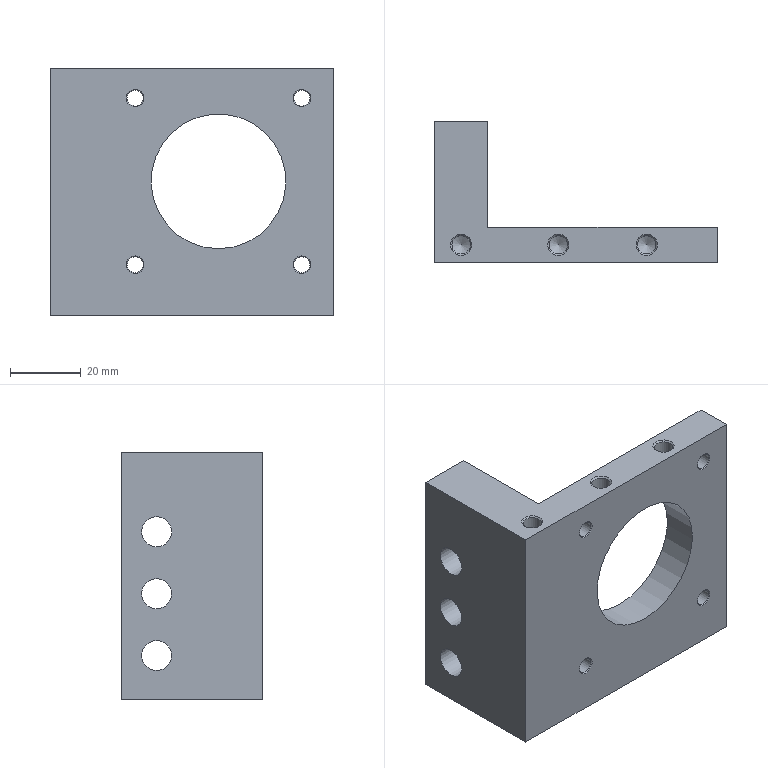Part | NX | features SIMPLE HOLE 8, SYMBOLIC_THREAD 7, DATUM_CSYS 6, SKETCH 5, HOLE PACKAGE 4, CBORE_HOLE 3, EXTRUDE 3 | 1 solid | 39 faces | box 80 x 40 x 70 mm | volume 69498 mm3 | cylinder 14 | cone 14 | plane 11 | commonest cylinder face diameters 4.5 x4 5.2 x3 8.5 x3 14 x3 38.1 x1
STEP:
#1=CARTESIAN_POINT('',(80.,10.,0.));
#2=VERTEX_POINT('',#1);
#3=CARTESIAN_POINT('',(15.,10.,0.));
#4=VERTEX_POINT('',#3);
#5=CARTESIAN_POINT('',(80.,10.,0.));
#6=DIRECTION('',(-1.,0.,0.));
#7=VECTOR('',#6,1000.);
#8=LINE('',#5,#7);
#9=EDGE_CURVE('',#2,#4,#8,.T.);
#10=ORIENTED_EDGE('',*,*,#9,.F.);
#11=CARTESIAN_POINT('',(80.,0.,0.));
#12=VERTEX_POINT('',#11);
#13=CARTESIAN_POINT('',(80.,0.,0.));
#14=DIRECTION('',(0.,-1.,0.));
#15=VECTOR('',#14,1000.);
#16=LINE('',#13,#15);
#17=EDGE_CURVE('',#12,#2,#16,.F.);
#18=ORIENTED_EDGE('',*,*,#17,.F.);
#19=CARTESIAN_POINT('',(0.,0.,0.));
#20=VERTEX_POINT('',#19);
#21=CARTESIAN_POINT('',(0.,0.,0.));
#22=DIRECTION('',(1.,0.,0.));
#23=VECTOR('',#22,1000.);
#24=LINE('',#21,#23);
#25=EDGE_CURVE('',#20,#12,#24,.T.);
#26=ORIENTED_EDGE('',*,*,#25,.F.);
#27=CARTESIAN_POINT('',(0.,40.,0.));
#28=VERTEX_POINT('',#27);
#29=CARTESIAN_POINT('',(0.,40.,0.));
#30=DIRECTION('',(0.,-1.,0.));
#31=VECTOR('',#30,1000.);
#32=LINE('',#29,#31);
#33=EDGE_CURVE('',#28,#20,#32,.T.);
#34=ORIENTED_EDGE('',*,*,#33,.F.);
#35=CARTESIAN_POINT('',(15.,40.,0.));
#36=VERTEX_POINT('',#35);
#37=CARTESIAN_POINT('',(0.,40.,0.));
#38=DIRECTION('',(-1.,0.,0.));
#39=VECTOR('',#38,1000.);
#40=LINE('',#37,#39);
#41=EDGE_CURVE('',#28,#36,#40,.F.);
#42=ORIENTED_EDGE('',*,*,#41,.T.);
#43=CARTESIAN_POINT('',(15.,40.,0.));
#44=DIRECTION('',(0.,-1.,0.));
#45=VECTOR('',#44,1000.);
#46=LINE('',#43,#45);
#47=EDGE_CURVE('',#36,#4,#46,.T.);
#48=ORIENTED_EDGE('',*,*,#47,.T.);
#49=EDGE_LOOP('',(#10,#18,#26,#34,#42,#48));
#50=FACE_BOUND('',#49,.T.);
#51=CARTESIAN_POINT('',(0.,0.,0.));
#52=DIRECTION('',(0.,0.,-1.));
#53=DIRECTION('',(1.,0.,0.));
#54=AXIS2_PLACEMENT_3D('',#51,#52,#53);
#55=PLANE('',#54);
#56=ADVANCED_FACE('',(#50),#55,.T.);
#57=CARTESIAN_POINT('',(80.,10.,70.));
#58=VERTEX_POINT('',#57);
#59=CARTESIAN_POINT('',(80.,10.,60.));
#60=DIRECTION('',(0.,0.,-1.));
#61=VECTOR('',#60,1000.);
#62=LINE('',#59,#61);
#63=EDGE_CURVE('',#58,#2,#62,.T.);
#64=ORIENTED_EDGE('',*,*,#63,.F.);
#65=CARTESIAN_POINT('',(80.,0.,70.));
#66=VERTEX_POINT('',#65);
#67=CARTESIAN_POINT('',(80.,0.,70.));
#68=DIRECTION('',(0.,1.,0.));
#69=VECTOR('',#68,1000.);
#70=LINE('',#67,#69);
#71=EDGE_CURVE('',#66,#58,#70,.T.);
#72=ORIENTED_EDGE('',*,*,#71,.F.);
#73=CARTESIAN_POINT('',(80.,0.,0.));
#74=DIRECTION('',(0.,0.,1.));
#75=VECTOR('',#74,1000.);
#76=LINE('',#73,#75);
#77=EDGE_CURVE('',#12,#66,#76,.T.);
#78=ORIENTED_EDGE('',*,*,#77,.F.);
#79=ORIENTED_EDGE('',*,*,#17,.T.);
#80=EDGE_LOOP('',(#64,#72,#78,#79));
#81=FACE_BOUND('',#80,.T.);
#82=CARTESIAN_POINT('',(80.,0.,0.));
#83=DIRECTION('',(1.,0.,0.));
#84=DIRECTION('',(0.,0.,1.));
#85=AXIS2_PLACEMENT_3D('',#82,#83,#84);
#86=PLANE('',#85);
#87=ADVANCED_FACE('',(#81),#86,.T.);
#88=CARTESIAN_POINT('',(47.5,0.,18.95));
#89=VERTEX_POINT('',#88);
#90=CARTESIAN_POINT('',(47.5,0.,38.));
#91=DIRECTION('',(0.,-1.,0.));
#92=DIRECTION('',(0.,0.,-1.));
#93=AXIS2_PLACEMENT_3D('',#90,#91,#92);
#94=CIRCLE('',#93,19.05);
#95=EDGE_CURVE('',#89,#89,#94,.T.);
#96=ORIENTED_EDGE('',*,*,#95,.T.);
#97=EDGE_LOOP('',(#96));
#98=FACE_BOUND('',#97,.T.);
#99=CARTESIAN_POINT('',(47.5,10.,18.95));
#100=VERTEX_POINT('',#99);
#101=CARTESIAN_POINT('',(47.5,10.,38.));
#102=DIRECTION('',(0.,-1.,0.));
#103=DIRECTION('',(0.,0.,-1.));
#104=AXIS2_PLACEMENT_3D('',#101,#102,#103);
#105=CIRCLE('',#104,19.05);
#106=EDGE_CURVE('',#100,#100,#105,.T.);
#107=ORIENTED_EDGE('',*,*,#106,.F.);
#108=EDGE_LOOP('',(#107));
#109=FACE_BOUND('',#108,.T.);
#110=CARTESIAN_POINT('',(47.5,15.,38.));
#111=DIRECTION('',(0.,-1.,0.));
#112=DIRECTION('',(0.,0.,-1.));
#113=AXIS2_PLACEMENT_3D('',#110,#111,#112);
#114=CYLINDRICAL_SURFACE('',#113,19.05);
#115=ADVANCED_FACE('',(#98,#109),#114,.F.);
#116=CARTESIAN_POINT('',(0.,40.,70.));
#117=VERTEX_POINT('',#116);
#118=CARTESIAN_POINT('',(0.,40.,0.));
#119=DIRECTION('',(0.,0.,1.));
#120=VECTOR('',#119,1000.);
#121=LINE('',#118,#120);
#122=EDGE_CURVE('',#28,#117,#121,.T.);
#123=ORIENTED_EDGE('',*,*,#122,.T.);
#124=CARTESIAN_POINT('',(15.,40.,70.));
#125=VERTEX_POINT('',#124);
#126=CARTESIAN_POINT('',(15.,40.,70.));
#127=DIRECTION('',(-1.,0.,0.));
#128=VECTOR('',#127,1000.);
#129=LINE('',#126,#128);
#130=EDGE_CURVE('',#125,#117,#129,.T.);
#131=ORIENTED_EDGE('',*,*,#130,.F.);
#132=CARTESIAN_POINT('',(15.,40.,0.));
#133=DIRECTION('',(0.,0.,1.));
#134=VECTOR('',#133,1000.);
#135=LINE('',#132,#134);
#136=EDGE_CURVE('',#36,#125,#135,.T.);
#137=ORIENTED_EDGE('',*,*,#136,.F.);
#138=ORIENTED_EDGE('',*,*,#41,.F.);
#139=EDGE_LOOP('',(#123,#131,#137,#138));
#140=FACE_BOUND('',#139,.T.);
#141=CARTESIAN_POINT('',(0.,40.,0.));
#142=DIRECTION('',(0.,-1.,0.));
#143=DIRECTION('',(0.,0.,1.));
#144=AXIS2_PLACEMENT_3D('',#141,#142,#143);
#145=PLANE('',#144);
#146=ADVANCED_FACE('',(#140),#145,.F.);
#147=CARTESIAN_POINT('',(15.,23.,47.5));
#148=VERTEX_POINT('',#147);
#149=CARTESIAN_POINT('',(15.,30.,47.5));
#150=DIRECTION('',(-1.,0.,0.));
#151=DIRECTION('',(0.,-1.,0.));
#152=AXIS2_PLACEMENT_3D('',#149,#150,#151);
#153=CIRCLE('',#152,7.);
#154=EDGE_CURVE('',#148,#148,#153,.T.);
#155=ORIENTED_EDGE('',*,*,#154,.T.);
#156=EDGE_LOOP('',(#155));
#157=FACE_BOUND('',#156,.T.);
#158=CARTESIAN_POINT('',(15.,23.,30.));
#159=VERTEX_POINT('',#158);
#160=CARTESIAN_POINT('',(15.,30.,30.));
#161=DIRECTION('',(-1.,0.,0.));
#162=DIRECTION('',(0.,-1.,0.));
#163=AXIS2_PLACEMENT_3D('',#160,#161,#162);
#164=CIRCLE('',#163,7.);
#165=EDGE_CURVE('',#159,#159,#164,.T.);
#166=ORIENTED_EDGE('',*,*,#165,.T.);
#167=EDGE_LOOP('',(#166));
#168=FACE_BOUND('',#167,.T.);
#169=CARTESIAN_POINT('',(15.,23.,12.5));
#170=VERTEX_POINT('',#169);
#171=CARTESIAN_POINT('',(15.,30.,12.5));
#172=DIRECTION('',(-1.,0.,0.));
#173=DIRECTION('',(0.,-1.,0.));
#174=AXIS2_PLACEMENT_3D('',#171,#172,#173);
#175=CIRCLE('',#174,7.);
#176=EDGE_CURVE('',#170,#170,#175,.T.);
#177=ORIENTED_EDGE('',*,*,#176,.T.);
#178=EDGE_LOOP('',(#177));
#179=FACE_BOUND('',#178,.T.);
#180=ORIENTED_EDGE('',*,*,#136,.T.);
#181=CARTESIAN_POINT('',(15.,10.,70.));
#182=VERTEX_POINT('',#181);
#183=CARTESIAN_POINT('',(15.,10.,70.));
#184=DIRECTION('',(0.,1.,0.));
#185=VECTOR('',#184,1000.);
#186=LINE('',#183,#185);
#187=EDGE_CURVE('',#182,#125,#186,.T.);
#188=ORIENTED_EDGE('',*,*,#187,.F.);
#189=CARTESIAN_POINT('',(15.,10.,0.));
#190=DIRECTION('',(0.,0.,1.));
#191=VECTOR('',#190,1000.);
#192=LINE('',#189,#191);
#193=EDGE_CURVE('',#4,#182,#192,.T.);
#194=ORIENTED_EDGE('',*,*,#193,.F.);
#195=ORIENTED_EDGE('',*,*,#47,.F.);
#196=EDGE_LOOP('',(#180,#188,#194,#195));
#197=FACE_BOUND('',#196,.T.);
#198=CARTESIAN_POINT('',(15.,40.,0.));
#199=DIRECTION('',(-1.,0.,0.));
#200=DIRECTION('',(0.,-1.,0.));
#201=AXIS2_PLACEMENT_3D('',#198,#199,#200);
#202=PLANE('',#201);
#203=ADVANCED_FACE('',(#157,#168,#179,#197),#202,.F.);
#204=CARTESIAN_POINT('',(0.,25.75,47.5));
#205=VERTEX_POINT('',#204);
#206=CARTESIAN_POINT('',(0.,30.,47.5));
#207=DIRECTION('',(-1.,0.,0.));
#208=DIRECTION('',(0.,-1.,0.));
#209=AXIS2_PLACEMENT_3D('',#206,#207,#208);
#210=CIRCLE('',#209,4.25);
#211=EDGE_CURVE('',#205,#205,#210,.T.);
#212=ORIENTED_EDGE('',*,*,#211,.F.);
#213=EDGE_LOOP('',(#212));
#214=FACE_BOUND('',#213,.T.);
#215=CARTESIAN_POINT('',(0.,25.75,30.));
#216=VERTEX_POINT('',#215);
#217=CARTESIAN_POINT('',(0.,30.,30.));
#218=DIRECTION('',(-1.,0.,0.));
#219=DIRECTION('',(0.,-1.,0.));
#220=AXIS2_PLACEMENT_3D('',#217,#218,#219);
#221=CIRCLE('',#220,4.25);
#222=EDGE_CURVE('',#216,#216,#221,.T.);
#223=ORIENTED_EDGE('',*,*,#222,.F.);
#224=EDGE_LOOP('',(#223));
#225=FACE_BOUND('',#224,.T.);
#226=CARTESIAN_POINT('',(0.,25.75,12.5));
#227=VERTEX_POINT('',#226);
#228=CARTESIAN_POINT('',(0.,30.,12.5));
#229=DIRECTION('',(-1.,0.,0.));
#230=DIRECTION('',(0.,-1.,0.));
#231=AXIS2_PLACEMENT_3D('',#228,#229,#230);
#232=CIRCLE('',#231,4.25);
#233=EDGE_CURVE('',#227,#227,#232,.T.);
#234=ORIENTED_EDGE('',*,*,#233,.F.);
#235=EDGE_LOOP('',(#234));
#236=FACE_BOUND('',#235,.T.);
#237=CARTESIAN_POINT('',(0.,0.,70.));
#238=VERTEX_POINT('',#237);
#239=CARTESIAN_POINT('',(0.,0.,0.));
#240=DIRECTION('',(0.,0.,1.));
#241=VECTOR('',#240,1000.);
#242=LINE('',#239,#241);
#243=EDGE_CURVE('',#20,#238,#242,.T.);
#244=ORIENTED_EDGE('',*,*,#243,.T.);
#245=CARTESIAN_POINT('',(0.,40.,70.));
#246=DIRECTION('',(0.,-1.,0.));
#247=VECTOR('',#246,1000.);
#248=LINE('',#245,#247);
#249=EDGE_CURVE('',#117,#238,#248,.T.);
#250=ORIENTED_EDGE('',*,*,#249,.F.);
#251=ORIENTED_EDGE('',*,*,#122,.F.);
#252=ORIENTED_EDGE('',*,*,#33,.T.);
#253=EDGE_LOOP('',(#244,#250,#251,#252));
#254=FACE_BOUND('',#253,.T.);
#255=CARTESIAN_POINT('',(0.,40.,0.));
#256=DIRECTION('',(-1.,0.,0.));
#257=DIRECTION('',(0.,-1.,0.));
#258=AXIS2_PLACEMENT_3D('',#255,#256,#257);
#259=PLANE('',#258);
#260=ADVANCED_FACE('',(#214,#225,#236,#254),#259,.T.);
#261=CARTESIAN_POINT('',(23.93,0.,11.93));
#262=VERTEX_POINT('',#261);
#263=CARTESIAN_POINT('',(23.93,0.,14.43));
#264=DIRECTION('',(0.,-1.,0.));
#265=DIRECTION('',(0.,0.,-1.));
#266=AXIS2_PLACEMENT_3D('',#263,#264,#265);
#267=CIRCLE('',#266,2.5);
#268=EDGE_CURVE('',#262,#262,#267,.F.);
#269=ORIENTED_EDGE('',*,*,#268,.T.);
#270=EDGE_LOOP('',(#269));
#271=FACE_BOUND('',#270,.T.);
#272=CARTESIAN_POINT('',(23.93,0.,59.07));
#273=VERTEX_POINT('',#272);
#274=CARTESIAN_POINT('',(23.93,0.,61.57));
#275=DIRECTION('',(0.,-1.,0.));
#276=DIRECTION('',(0.,0.,-1.));
#277=AXIS2_PLACEMENT_3D('',#274,#275,#276);
#278=CIRCLE('',#277,2.5);
#279=EDGE_CURVE('',#273,#273,#278,.F.);
#280=ORIENTED_EDGE('',*,*,#279,.T.);
#281=EDGE_LOOP('',(#280));
#282=FACE_BOUND('',#281,.T.);
#283=CARTESIAN_POINT('',(71.07,0.,59.07));
#284=VERTEX_POINT('',#283);
#285=CARTESIAN_POINT('',(71.07,0.,61.57));
#286=DIRECTION('',(0.,-1.,0.));
#287=DIRECTION('',(0.,0.,-1.));
#288=AXIS2_PLACEMENT_3D('',#285,#286,#287);
#289=CIRCLE('',#288,2.5);
#290=EDGE_CURVE('',#284,#284,#289,.F.);
#291=ORIENTED_EDGE('',*,*,#290,.T.);
#292=EDGE_LOOP('',(#291));
#293=FACE_BOUND('',#292,.T.);
#294=CARTESIAN_POINT('',(71.07,0.,11.93));
#295=VERTEX_POINT('',#294);
#296=CARTESIAN_POINT('',(71.07,0.,14.43));
#297=DIRECTION('',(0.,-1.,0.));
#298=DIRECTION('',(0.,0.,-1.));
#299=AXIS2_PLACEMENT_3D('',#296,#297,#298);
#300=CIRCLE('',#299,2.5);
#301=EDGE_CURVE('',#295,#295,#300,.F.);
#302=ORIENTED_EDGE('',*,*,#301,.T.);
#303=EDGE_LOOP('',(#302));
#304=FACE_BOUND('',#303,.T.);
#305=ORIENTED_EDGE('',*,*,#95,.F.);
#306=EDGE_LOOP('',(#305));
#307=FACE_BOUND('',#306,.T.);
#308=ORIENTED_EDGE('',*,*,#77,.T.);
#309=CARTESIAN_POINT('',(0.,0.,70.));
#310=DIRECTION('',(1.,0.,0.));
#311=VECTOR('',#310,1000.);
#312=LINE('',#309,#311);
#313=EDGE_CURVE('',#238,#66,#312,.T.);
#314=ORIENTED_EDGE('',*,*,#313,.F.);
#315=ORIENTED_EDGE('',*,*,#243,.F.);
#316=ORIENTED_EDGE('',*,*,#25,.T.);
#317=EDGE_LOOP('',(#308,#314,#315,#316));
#318=FACE_BOUND('',#317,.T.);
#319=CARTESIAN_POINT('',(0.,0.,0.));
#320=DIRECTION('',(0.,-1.,0.));
#321=DIRECTION('',(0.,0.,-1.));
#322=AXIS2_PLACEMENT_3D('',#319,#320,#321);
#323=PLANE('',#322);
#324=ADVANCED_FACE('',(#271,#282,#293,#304,#307,#318),#323,.T.);
#325=CARTESIAN_POINT('',(23.93,10.,11.93));
#326=VERTEX_POINT('',#325);
#327=CARTESIAN_POINT('',(23.93,10.,14.43));
#328=DIRECTION('',(0.,-1.,0.));
#329=DIRECTION('',(0.,0.,-1.));
#330=AXIS2_PLACEMENT_3D('',#327,#328,#329);
#331=CIRCLE('',#330,2.5);
#332=EDGE_CURVE('',#326,#326,#331,.T.);
#333=ORIENTED_EDGE('',*,*,#332,.T.);
#334=EDGE_LOOP('',(#333));
#335=FACE_BOUND('',#334,.T.);
#336=CARTESIAN_POINT('',(23.93,10.,59.07));
#337=VERTEX_POINT('',#336);
#338=CARTESIAN_POINT('',(23.93,10.,61.57));
#339=DIRECTION('',(0.,-1.,0.));
#340=DIRECTION('',(0.,0.,-1.));
#341=AXIS2_PLACEMENT_3D('',#338,#339,#340);
#342=CIRCLE('',#341,2.5);
#343=EDGE_CURVE('',#337,#337,#342,.T.);
#344=ORIENTED_EDGE('',*,*,#343,.T.);
#345=EDGE_LOOP('',(#344));
#346=FACE_BOUND('',#345,.T.);
#347=CARTESIAN_POINT('',(71.07,10.,59.07));
#348=VERTEX_POINT('',#347);
#349=CARTESIAN_POINT('',(71.07,10.,61.57));
#350=DIRECTION('',(0.,-1.,0.));
#351=DIRECTION('',(0.,0.,-1.));
#352=AXIS2_PLACEMENT_3D('',#349,#350,#351);
#353=CIRCLE('',#352,2.5);
#354=EDGE_CURVE('',#348,#348,#353,.T.);
#355=ORIENTED_EDGE('',*,*,#354,.T.);
#356=EDGE_LOOP('',(#355));
#357=FACE_BOUND('',#356,.T.);
#358=CARTESIAN_POINT('',(71.07,10.,11.93));
#359=VERTEX_POINT('',#358);
#360=CARTESIAN_POINT('',(71.07,10.,14.43));
#361=DIRECTION('',(0.,-1.,0.));
#362=DIRECTION('',(0.,0.,-1.));
#363=AXIS2_PLACEMENT_3D('',#360,#361,#362);
#364=CIRCLE('',#363,2.5);
#365=EDGE_CURVE('',#359,#359,#364,.T.);
#366=ORIENTED_EDGE('',*,*,#365,.T.);
#367=EDGE_LOOP('',(#366));
#368=FACE_BOUND('',#367,.T.);
#369=ORIENTED_EDGE('',*,*,#193,.T.);
#370=CARTESIAN_POINT('',(80.,10.,70.));
#371=DIRECTION('',(-1.,0.,0.));
#372=VECTOR('',#371,1000.);
#373=LINE('',#370,#372);
#374=EDGE_CURVE('',#58,#182,#373,.T.);
#375=ORIENTED_EDGE('',*,*,#374,.F.);
#376=ORIENTED_EDGE('',*,*,#63,.T.);
#377=ORIENTED_EDGE('',*,*,#9,.T.);
#378=EDGE_LOOP('',(#369,#375,#376,#377));
#379=FACE_BOUND('',#378,.T.);
#380=ORIENTED_EDGE('',*,*,#106,.T.);
#381=EDGE_LOOP('',(#380));
#382=FACE_BOUND('',#381,.T.);
#383=CARTESIAN_POINT('',(47.5,10.,38.));
#384=DIRECTION('',(0.,-1.,0.));
#385=DIRECTION('',(0.,0.,-1.));
#386=AXIS2_PLACEMENT_3D('',#383,#384,#385);
#387=PLANE('',#386);
#388=ADVANCED_FACE('',(#335,#346,#357,#368,#379,#382),#387,.F.);
#389=CARTESIAN_POINT('',(63.,5.,70.));
#390=VERTEX_POINT('',#389);
#391=CARTESIAN_POINT('',(60.,5.,70.));
#392=DIRECTION('',(0.,0.,1.));
#393=DIRECTION('',(1.,0.,0.));
#394=AXIS2_PLACEMENT_3D('',#391,#392,#393);
#395=CIRCLE('',#394,3.);
#396=EDGE_CURVE('',#390,#390,#395,.F.);
#397=ORIENTED_EDGE('',*,*,#396,.T.);
#398=EDGE_LOOP('',(#397));
#399=FACE_BOUND('',#398,.T.);
#400=CARTESIAN_POINT('',(38.,5.,70.));
#401=VERTEX_POINT('',#400);
#402=CARTESIAN_POINT('',(35.,5.,70.));
#403=DIRECTION('',(0.,0.,1.));
#404=DIRECTION('',(1.,0.,0.));
#405=AXIS2_PLACEMENT_3D('',#402,#403,#404);
#406=CIRCLE('',#405,3.);
#407=EDGE_CURVE('',#401,#401,#406,.F.);
#408=ORIENTED_EDGE('',*,*,#407,.T.);
#409=EDGE_LOOP('',(#408));
#410=FACE_BOUND('',#409,.T.);
#411=CARTESIAN_POINT('',(10.5,5.,70.));
#412=VERTEX_POINT('',#411);
#413=CARTESIAN_POINT('',(7.5,5.,70.));
#414=DIRECTION('',(0.,0.,1.));
#415=DIRECTION('',(1.,0.,0.));
#416=AXIS2_PLACEMENT_3D('',#413,#414,#415);
#417=CIRCLE('',#416,3.);
#418=EDGE_CURVE('',#412,#412,#417,.F.);
#419=ORIENTED_EDGE('',*,*,#418,.T.);
#420=EDGE_LOOP('',(#419));
#421=FACE_BOUND('',#420,.T.);
#422=ORIENTED_EDGE('',*,*,#249,.T.);
#423=ORIENTED_EDGE('',*,*,#313,.T.);
#424=ORIENTED_EDGE('',*,*,#71,.T.);
#425=ORIENTED_EDGE('',*,*,#374,.T.);
#426=ORIENTED_EDGE('',*,*,#187,.T.);
#427=ORIENTED_EDGE('',*,*,#130,.T.);
#428=EDGE_LOOP('',(#422,#423,#424,#425,#426,#427));
#429=FACE_BOUND('',#428,.T.);
#430=CARTESIAN_POINT('',(0.,0.,70.));
#431=DIRECTION('',(0.,0.,1.));
#432=DIRECTION('',(1.,0.,0.));
#433=AXIS2_PLACEMENT_3D('',#430,#431,#432);
#434=PLANE('',#433);
#435=ADVANCED_FACE('',(#399,#410,#421,#429),#434,.T.);
#436=CARTESIAN_POINT('',(71.07,0.25,12.18));
#437=VERTEX_POINT('',#436);
#438=CARTESIAN_POINT('',(71.07,0.25,14.43));
#439=DIRECTION('',(0.,-1.,0.));
#440=DIRECTION('',(0.,0.,-1.));
#441=AXIS2_PLACEMENT_3D('',#438,#439,#440);
#442=CIRCLE('',#441,2.25);
#443=EDGE_CURVE('',#437,#437,#442,.T.);
#444=ORIENTED_EDGE('',*,*,#443,.T.);
#445=EDGE_LOOP('',(#444));
#446=FACE_BOUND('',#445,.T.);
#447=CARTESIAN_POINT('',(71.07,9.75,12.18));
#448=VERTEX_POINT('',#447);
#449=CARTESIAN_POINT('',(71.07,9.75,14.43));
#450=DIRECTION('',(0.,-1.,0.));
#451=DIRECTION('',(0.,0.,-1.));
#452=AXIS2_PLACEMENT_3D('',#449,#450,#451);
#453=CIRCLE('',#452,2.25);
#454=EDGE_CURVE('',#448,#448,#453,.F.);
#455=ORIENTED_EDGE('',*,*,#454,.T.);
#456=EDGE_LOOP('',(#455));
#457=FACE_BOUND('',#456,.T.);
#458=CARTESIAN_POINT('',(71.07,10.,14.43));
#459=DIRECTION('',(0.,-1.,0.));
#460=DIRECTION('',(0.,0.,-1.));
#461=AXIS2_PLACEMENT_3D('',#458,#459,#460);
#462=CYLINDRICAL_SURFACE('',#461,2.25);
#463=ADVANCED_FACE('',(#446,#457),#462,.F.);
#464=ORIENTED_EDGE('',*,*,#454,.F.);
#465=EDGE_LOOP('',(#464));
#466=FACE_BOUND('',#465,.T.);
#467=ORIENTED_EDGE('',*,*,#365,.F.);
#468=EDGE_LOOP('',(#467));
#469=FACE_BOUND('',#468,.T.);
#470=CARTESIAN_POINT('',(71.07,10.,14.43));
#471=DIRECTION('',(0.,1.,0.));
#472=DIRECTION('',(0.,0.,1.));
#473=AXIS2_PLACEMENT_3D('',#470,#471,#472);
#474=CONICAL_SURFACE('',#473,2.5,0.7854);
#475=ADVANCED_FACE('',(#466,#469),#474,.F.);
#476=ORIENTED_EDGE('',*,*,#301,.F.);
#477=EDGE_LOOP('',(#476));
#478=FACE_BOUND('',#477,.T.);
#479=ORIENTED_EDGE('',*,*,#443,.F.);
#480=EDGE_LOOP('',(#479));
#481=FACE_BOUND('',#480,.T.);
#482=CARTESIAN_POINT('',(71.07,0.25,14.43));
#483=DIRECTION('',(0.,-1.,0.));
#484=DIRECTION('',(0.,0.,-1.));
#485=AXIS2_PLACEMENT_3D('',#482,#483,#484);
#486=CONICAL_SURFACE('',#485,2.25,0.7854);
#487=ADVANCED_FACE('',(#478,#481),#486,.F.);
#488=CARTESIAN_POINT('',(71.07,0.25,59.32));
#489=VERTEX_POINT('',#488);
#490=CARTESIAN_POINT('',(71.07,0.25,61.57));
#491=DIRECTION('',(0.,-1.,0.));
#492=DIRECTION('',(0.,0.,-1.));
#493=AXIS2_PLACEMENT_3D('',#490,#491,#492);
#494=CIRCLE('',#493,2.25);
#495=EDGE_CURVE('',#489,#489,#494,.T.);
#496=ORIENTED_EDGE('',*,*,#495,.T.);
#497=EDGE_LOOP('',(#496));
#498=FACE_BOUND('',#497,.T.);
#499=CARTESIAN_POINT('',(71.07,9.75,59.32));
#500=VERTEX_POINT('',#499);
#501=CARTESIAN_POINT('',(71.07,9.75,61.57));
#502=DIRECTION('',(0.,-1.,0.));
#503=DIRECTION('',(0.,0.,-1.));
#504=AXIS2_PLACEMENT_3D('',#501,#502,#503);
#505=CIRCLE('',#504,2.25);
#506=EDGE_CURVE('',#500,#500,#505,.F.);
#507=ORIENTED_EDGE('',*,*,#506,.T.);
#508=EDGE_LOOP('',(#507));
#509=FACE_BOUND('',#508,.T.);
#510=CARTESIAN_POINT('',(71.07,10.,61.57));
#511=DIRECTION('',(0.,-1.,0.));
#512=DIRECTION('',(0.,0.,-1.));
#513=AXIS2_PLACEMENT_3D('',#510,#511,#512);
#514=CYLINDRICAL_SURFACE('',#513,2.25);
#515=ADVANCED_FACE('',(#498,#509),#514,.F.);
#516=ORIENTED_EDGE('',*,*,#506,.F.);
#517=EDGE_LOOP('',(#516));
#518=FACE_BOUND('',#517,.T.);
#519=ORIENTED_EDGE('',*,*,#354,.F.);
#520=EDGE_LOOP('',(#519));
#521=FACE_BOUND('',#520,.T.);
#522=CARTESIAN_POINT('',(71.07,10.,61.57));
#523=DIRECTION('',(0.,1.,0.));
#524=DIRECTION('',(0.,0.,1.));
#525=AXIS2_PLACEMENT_3D('',#522,#523,#524);
#526=CONICAL_SURFACE('',#525,2.5,0.7854);
#527=ADVANCED_FACE('',(#518,#521),#526,.F.);
#528=ORIENTED_EDGE('',*,*,#290,.F.);
#529=EDGE_LOOP('',(#528));
#530=FACE_BOUND('',#529,.T.);
#531=ORIENTED_EDGE('',*,*,#495,.F.);
#532=EDGE_LOOP('',(#531));
#533=FACE_BOUND('',#532,.T.);
#534=CARTESIAN_POINT('',(71.07,0.25,61.57));
#535=DIRECTION('',(0.,-1.,0.));
#536=DIRECTION('',(0.,0.,-1.));
#537=AXIS2_PLACEMENT_3D('',#534,#535,#536);
#538=CONICAL_SURFACE('',#537,2.25,0.7854);
#539=ADVANCED_FACE('',(#530,#533),#538,.F.);
#540=CARTESIAN_POINT('',(23.93,0.25,59.32));
#541=VERTEX_POINT('',#540);
#542=CARTESIAN_POINT('',(23.93,0.25,61.57));
#543=DIRECTION('',(0.,-1.,0.));
#544=DIRECTION('',(0.,0.,-1.));
#545=AXIS2_PLACEMENT_3D('',#542,#543,#544);
#546=CIRCLE('',#545,2.25);
#547=EDGE_CURVE('',#541,#541,#546,.T.);
#548=ORIENTED_EDGE('',*,*,#547,.T.);
#549=EDGE_LOOP('',(#548));
#550=FACE_BOUND('',#549,.T.);
#551=CARTESIAN_POINT('',(23.93,9.75,59.32));
#552=VERTEX_POINT('',#551);
#553=CARTESIAN_POINT('',(23.93,9.75,61.57));
#554=DIRECTION('',(0.,-1.,0.));
#555=DIRECTION('',(0.,0.,-1.));
#556=AXIS2_PLACEMENT_3D('',#553,#554,#555);
#557=CIRCLE('',#556,2.25);
#558=EDGE_CURVE('',#552,#552,#557,.F.);
#559=ORIENTED_EDGE('',*,*,#558,.T.);
#560=EDGE_LOOP('',(#559));
#561=FACE_BOUND('',#560,.T.);
#562=CARTESIAN_POINT('',(23.93,10.,61.57));
#563=DIRECTION('',(0.,-1.,0.));
#564=DIRECTION('',(0.,0.,-1.));
#565=AXIS2_PLACEMENT_3D('',#562,#563,#564);
#566=CYLINDRICAL_SURFACE('',#565,2.25);
#567=ADVANCED_FACE('',(#550,#561),#566,.F.);
#568=ORIENTED_EDGE('',*,*,#558,.F.);
#569=EDGE_LOOP('',(#568));
#570=FACE_BOUND('',#569,.T.);
#571=ORIENTED_EDGE('',*,*,#343,.F.);
#572=EDGE_LOOP('',(#571));
#573=FACE_BOUND('',#572,.T.);
#574=CARTESIAN_POINT('',(23.93,10.,61.57));
#575=DIRECTION('',(0.,1.,0.));
#576=DIRECTION('',(0.,0.,1.));
#577=AXIS2_PLACEMENT_3D('',#574,#575,#576);
#578=CONICAL_SURFACE('',#577,2.5,0.7854);
#579=ADVANCED_FACE('',(#570,#573),#578,.F.);
#580=ORIENTED_EDGE('',*,*,#279,.F.);
#581=EDGE_LOOP('',(#580));
#582=FACE_BOUND('',#581,.T.);
#583=ORIENTED_EDGE('',*,*,#547,.F.);
#584=EDGE_LOOP('',(#583));
#585=FACE_BOUND('',#584,.T.);
#586=CARTESIAN_POINT('',(23.93,0.25,61.57));
#587=DIRECTION('',(0.,-1.,0.));
#588=DIRECTION('',(0.,0.,-1.));
#589=AXIS2_PLACEMENT_3D('',#586,#587,#588);
#590=CONICAL_SURFACE('',#589,2.25,0.7854);
#591=ADVANCED_FACE('',(#582,#585),#590,.F.);
#592=CARTESIAN_POINT('',(23.93,0.25,12.18));
#593=VERTEX_POINT('',#592);
#594=CARTESIAN_POINT('',(23.93,0.25,14.43));
#595=DIRECTION('',(0.,-1.,0.));
#596=DIRECTION('',(0.,0.,-1.));
#597=AXIS2_PLACEMENT_3D('',#594,#595,#596);
#598=CIRCLE('',#597,2.25);
#599=EDGE_CURVE('',#593,#593,#598,.T.);
#600=ORIENTED_EDGE('',*,*,#599,.T.);
#601=EDGE_LOOP('',(#600));
#602=FACE_BOUND('',#601,.T.);
#603=CARTESIAN_POINT('',(23.93,9.75,12.18));
#604=VERTEX_POINT('',#603);
#605=CARTESIAN_POINT('',(23.93,9.75,14.43));
#606=DIRECTION('',(0.,-1.,0.));
#607=DIRECTION('',(0.,0.,-1.));
#608=AXIS2_PLACEMENT_3D('',#605,#606,#607);
#609=CIRCLE('',#608,2.25);
#610=EDGE_CURVE('',#604,#604,#609,.F.);
#611=ORIENTED_EDGE('',*,*,#610,.T.);
#612=EDGE_LOOP('',(#611));
#613=FACE_BOUND('',#612,.T.);
#614=CARTESIAN_POINT('',(23.93,10.,14.43));
#615=DIRECTION('',(0.,-1.,0.));
#616=DIRECTION('',(0.,0.,-1.));
#617=AXIS2_PLACEMENT_3D('',#614,#615,#616);
#618=CYLINDRICAL_SURFACE('',#617,2.25);
#619=ADVANCED_FACE('',(#602,#613),#618,.F.);
#620=ORIENTED_EDGE('',*,*,#610,.F.);
#621=EDGE_LOOP('',(#620));
#622=FACE_BOUND('',#621,.T.);
#623=ORIENTED_EDGE('',*,*,#332,.F.);
#624=EDGE_LOOP('',(#623));
#625=FACE_BOUND('',#624,.T.);
#626=CARTESIAN_POINT('',(23.93,10.,14.43));
#627=DIRECTION('',(0.,1.,0.));
#628=DIRECTION('',(0.,0.,1.));
#629=AXIS2_PLACEMENT_3D('',#626,#627,#628);
#630=CONICAL_SURFACE('',#629,2.5,0.7854);
#631=ADVANCED_FACE('',(#622,#625),#630,.F.);
#632=ORIENTED_EDGE('',*,*,#268,.F.);
#633=EDGE_LOOP('',(#632));
#634=FACE_BOUND('',#633,.T.);
#635=ORIENTED_EDGE('',*,*,#599,.F.);
#636=EDGE_LOOP('',(#635));
#637=FACE_BOUND('',#636,.T.);
#638=CARTESIAN_POINT('',(23.93,0.25,14.43));
#639=DIRECTION('',(0.,-1.,0.));
#640=DIRECTION('',(0.,0.,-1.));
#641=AXIS2_PLACEMENT_3D('',#638,#639,#640);
#642=CONICAL_SURFACE('',#641,2.25,0.7854);
#643=ADVANCED_FACE('',(#634,#637),#642,.F.);
#644=CARTESIAN_POINT('',(4.9,5.,56.));
#645=VERTEX_POINT('',#644);
#646=CARTESIAN_POINT('',(7.5,5.,56.));
#647=DIRECTION('',(0.,0.,-1.));
#648=DIRECTION('',(-1.,0.,0.));
#649=AXIS2_PLACEMENT_3D('',#646,#647,#648);
#650=CIRCLE('',#649,2.6);
#651=EDGE_CURVE('',#645,#645,#650,.F.);
#652=ORIENTED_EDGE('',*,*,#651,.T.);
#653=EDGE_LOOP('',(#652));
#654=FACE_BOUND('',#653,.T.);
#655=CARTESIAN_POINT('',(7.5,5.,54.438));
#656=VERTEX_POINT('',#655);
#657=VERTEX_LOOP('',#656);
#658=FACE_BOUND('',#657,.T.);
#659=CARTESIAN_POINT('',(7.5,5.,56.));
#660=DIRECTION('',(0.,0.,1.));
#661=DIRECTION('',(1.,0.,0.));
#662=AXIS2_PLACEMENT_3D('',#659,#660,#661);
#663=CONICAL_SURFACE('',#662,2.6,1.03);
#664=ADVANCED_FACE('',(#654,#658),#663,.F.);
#665=CARTESIAN_POINT('',(10.1,5.,69.6));
#666=VERTEX_POINT('',#665);
#667=CARTESIAN_POINT('',(7.5,5.,69.6));
#668=DIRECTION('',(0.,0.,1.));
#669=DIRECTION('',(1.,0.,0.));
#670=AXIS2_PLACEMENT_3D('',#667,#668,#669);
#671=CIRCLE('',#670,2.6);
#672=EDGE_CURVE('',#666,#666,#671,.T.);
#673=ORIENTED_EDGE('',*,*,#672,.T.);
#674=EDGE_LOOP('',(#673));
#675=FACE_BOUND('',#674,.T.);
#676=ORIENTED_EDGE('',*,*,#651,.F.);
#677=EDGE_LOOP('',(#676));
#678=FACE_BOUND('',#677,.T.);
#679=CARTESIAN_POINT('',(7.5,5.,70.));
#680=DIRECTION('',(0.,0.,-1.));
#681=DIRECTION('',(-1.,0.,0.));
#682=AXIS2_PLACEMENT_3D('',#679,#680,#681);
#683=CYLINDRICAL_SURFACE('',#682,2.6);
#684=ADVANCED_FACE('',(#675,#678),#683,.F.);
#685=ORIENTED_EDGE('',*,*,#672,.F.);
#686=EDGE_LOOP('',(#685));
#687=FACE_BOUND('',#686,.T.);
#688=ORIENTED_EDGE('',*,*,#418,.F.);
#689=EDGE_LOOP('',(#688));
#690=FACE_BOUND('',#689,.T.);
#691=CARTESIAN_POINT('',(7.5,5.,70.));
#692=DIRECTION('',(0.,0.,1.));
#693=DIRECTION('',(1.,0.,0.));
#694=AXIS2_PLACEMENT_3D('',#691,#692,#693);
#695=CONICAL_SURFACE('',#694,3.,0.7854);
#696=ADVANCED_FACE('',(#687,#690),#695,.F.);
#697=CARTESIAN_POINT('',(32.4,5.,56.));
#698=VERTEX_POINT('',#697);
#699=CARTESIAN_POINT('',(35.,5.,56.));
#700=DIRECTION('',(0.,0.,-1.));
#701=DIRECTION('',(-1.,0.,0.));
#702=AXIS2_PLACEMENT_3D('',#699,#700,#701);
#703=CIRCLE('',#702,2.6);
#704=EDGE_CURVE('',#698,#698,#703,.F.);
#705=ORIENTED_EDGE('',*,*,#704,.T.);
#706=EDGE_LOOP('',(#705));
#707=FACE_BOUND('',#706,.T.);
#708=CARTESIAN_POINT('',(35.,5.,54.438));
#709=VERTEX_POINT('',#708);
#710=VERTEX_LOOP('',#709);
#711=FACE_BOUND('',#710,.T.);
#712=CARTESIAN_POINT('',(35.,5.,56.));
#713=DIRECTION('',(0.,0.,1.));
#714=DIRECTION('',(1.,0.,0.));
#715=AXIS2_PLACEMENT_3D('',#712,#713,#714);
#716=CONICAL_SURFACE('',#715,2.6,1.03);
#717=ADVANCED_FACE('',(#707,#711),#716,.F.);
#718=CARTESIAN_POINT('',(37.6,5.,69.6));
#719=VERTEX_POINT('',#718);
#720=CARTESIAN_POINT('',(35.,5.,69.6));
#721=DIRECTION('',(0.,0.,1.));
#722=DIRECTION('',(1.,0.,0.));
#723=AXIS2_PLACEMENT_3D('',#720,#721,#722);
#724=CIRCLE('',#723,2.6);
#725=EDGE_CURVE('',#719,#719,#724,.T.);
#726=ORIENTED_EDGE('',*,*,#725,.T.);
#727=EDGE_LOOP('',(#726));
#728=FACE_BOUND('',#727,.T.);
#729=ORIENTED_EDGE('',*,*,#704,.F.);
#730=EDGE_LOOP('',(#729));
#731=FACE_BOUND('',#730,.T.);
#732=CARTESIAN_POINT('',(35.,5.,70.));
#733=DIRECTION('',(0.,0.,-1.));
#734=DIRECTION('',(-1.,0.,0.));
#735=AXIS2_PLACEMENT_3D('',#732,#733,#734);
#736=CYLINDRICAL_SURFACE('',#735,2.6);
#737=ADVANCED_FACE('',(#728,#731),#736,.F.);
#738=ORIENTED_EDGE('',*,*,#725,.F.);
#739=EDGE_LOOP('',(#738));
#740=FACE_BOUND('',#739,.T.);
#741=ORIENTED_EDGE('',*,*,#407,.F.);
#742=EDGE_LOOP('',(#741));
#743=FACE_BOUND('',#742,.T.);
#744=CARTESIAN_POINT('',(35.,5.,70.));
#745=DIRECTION('',(0.,0.,1.));
#746=DIRECTION('',(1.,0.,0.));
#747=AXIS2_PLACEMENT_3D('',#744,#745,#746);
#748=CONICAL_SURFACE('',#747,3.,0.7854);
#749=ADVANCED_FACE('',(#740,#743),#748,.F.);
#750=CARTESIAN_POINT('',(57.4,5.,56.));
#751=VERTEX_POINT('',#750);
#752=CARTESIAN_POINT('',(60.,5.,56.));
#753=DIRECTION('',(0.,0.,-1.));
#754=DIRECTION('',(-1.,0.,0.));
#755=AXIS2_PLACEMENT_3D('',#752,#753,#754);
#756=CIRCLE('',#755,2.6);
#757=EDGE_CURVE('',#751,#751,#756,.F.);
#758=ORIENTED_EDGE('',*,*,#757,.T.);
#759=EDGE_LOOP('',(#758));
#760=FACE_BOUND('',#759,.T.);
#761=CARTESIAN_POINT('',(60.,5.,54.438));
#762=VERTEX_POINT('',#761);
#763=VERTEX_LOOP('',#762);
#764=FACE_BOUND('',#763,.T.);
#765=CARTESIAN_POINT('',(60.,5.,56.));
#766=DIRECTION('',(0.,0.,1.));
#767=DIRECTION('',(1.,0.,0.));
#768=AXIS2_PLACEMENT_3D('',#765,#766,#767);
#769=CONICAL_SURFACE('',#768,2.6,1.03);
#770=ADVANCED_FACE('',(#760,#764),#769,.F.);
#771=CARTESIAN_POINT('',(62.6,5.,69.6));
#772=VERTEX_POINT('',#771);
#773=CARTESIAN_POINT('',(60.,5.,69.6));
#774=DIRECTION('',(0.,0.,1.));
#775=DIRECTION('',(1.,0.,0.));
#776=AXIS2_PLACEMENT_3D('',#773,#774,#775);
#777=CIRCLE('',#776,2.6);
#778=EDGE_CURVE('',#772,#772,#777,.T.);
#779=ORIENTED_EDGE('',*,*,#778,.T.);
#780=EDGE_LOOP('',(#779));
#781=FACE_BOUND('',#780,.T.);
#782=ORIENTED_EDGE('',*,*,#757,.F.);
#783=EDGE_LOOP('',(#782));
#784=FACE_BOUND('',#783,.T.);
#785=CARTESIAN_POINT('',(60.,5.,70.));
#786=DIRECTION('',(0.,0.,-1.));
#787=DIRECTION('',(-1.,0.,0.));
#788=AXIS2_PLACEMENT_3D('',#785,#786,#787);
#789=CYLINDRICAL_SURFACE('',#788,2.6);
#790=ADVANCED_FACE('',(#781,#784),#789,.F.);
#791=ORIENTED_EDGE('',*,*,#778,.F.);
#792=EDGE_LOOP('',(#791));
#793=FACE_BOUND('',#792,.T.);
#794=ORIENTED_EDGE('',*,*,#396,.F.);
#795=EDGE_LOOP('',(#794));
#796=FACE_BOUND('',#795,.T.);
#797=CARTESIAN_POINT('',(60.,5.,70.));
#798=DIRECTION('',(0.,0.,1.));
#799=DIRECTION('',(1.,0.,0.));
#800=AXIS2_PLACEMENT_3D('',#797,#798,#799);
#801=CONICAL_SURFACE('',#800,3.,0.7854);
#802=ADVANCED_FACE('',(#793,#796),#801,.F.);
#803=ORIENTED_EDGE('',*,*,#233,.T.);
#804=EDGE_LOOP('',(#803));
#805=FACE_BOUND('',#804,.T.);
#806=CARTESIAN_POINT('',(6.5,25.75,12.5));
#807=VERTEX_POINT('',#806);
#808=CARTESIAN_POINT('',(6.5,30.,12.5));
#809=DIRECTION('',(-1.,0.,0.));
#810=DIRECTION('',(0.,-1.,0.));
#811=AXIS2_PLACEMENT_3D('',#808,#809,#810);
#812=CIRCLE('',#811,4.25);
#813=EDGE_CURVE('',#807,#807,#812,.F.);
#814=ORIENTED_EDGE('',*,*,#813,.T.);
#815=EDGE_LOOP('',(#814));
#816=FACE_BOUND('',#815,.T.);
#817=CARTESIAN_POINT('',(-35.,30.,12.5));
#818=DIRECTION('',(-1.,0.,0.));
#819=DIRECTION('',(0.,-1.,0.));
#820=AXIS2_PLACEMENT_3D('',#817,#818,#819);
#821=CYLINDRICAL_SURFACE('',#820,4.25);
#822=ADVANCED_FACE('',(#805,#816),#821,.F.);
#823=ORIENTED_EDGE('',*,*,#813,.F.);
#824=EDGE_LOOP('',(#823));
#825=FACE_BOUND('',#824,.T.);
#826=CARTESIAN_POINT('',(6.5,23.,12.5));
#827=VERTEX_POINT('',#826);
#828=CARTESIAN_POINT('',(6.5,30.,12.5));
#829=DIRECTION('',(-1.,0.,0.));
#830=DIRECTION('',(0.,-1.,0.));
#831=AXIS2_PLACEMENT_3D('',#828,#829,#830);
#832=CIRCLE('',#831,7.);
#833=EDGE_CURVE('',#827,#827,#832,.F.);
#834=ORIENTED_EDGE('',*,*,#833,.T.);
#835=EDGE_LOOP('',(#834));
#836=FACE_BOUND('',#835,.T.);
#837=CARTESIAN_POINT('',(6.5,30.,12.5));
#838=DIRECTION('',(-1.,0.,0.));
#839=DIRECTION('',(0.,-1.,0.));
#840=AXIS2_PLACEMENT_3D('',#837,#838,#839);
#841=PLANE('',#840);
#842=ADVANCED_FACE('',(#825,#836),#841,.F.);
#843=ORIENTED_EDGE('',*,*,#833,.F.);
#844=EDGE_LOOP('',(#843));
#845=FACE_BOUND('',#844,.T.);
#846=ORIENTED_EDGE('',*,*,#176,.F.);
#847=EDGE_LOOP('',(#846));
#848=FACE_BOUND('',#847,.T.);
#849=CARTESIAN_POINT('',(15.,30.,12.5));
#850=DIRECTION('',(-1.,0.,0.));
#851=DIRECTION('',(0.,-1.,0.));
#852=AXIS2_PLACEMENT_3D('',#849,#850,#851);
#853=CYLINDRICAL_SURFACE('',#852,7.);
#854=ADVANCED_FACE('',(#845,#848),#853,.F.);
#855=ORIENTED_EDGE('',*,*,#222,.T.);
#856=EDGE_LOOP('',(#855));
#857=FACE_BOUND('',#856,.T.);
#858=CARTESIAN_POINT('',(6.5,25.75,30.));
#859=VERTEX_POINT('',#858);
#860=CARTESIAN_POINT('',(6.5,30.,30.));
#861=DIRECTION('',(-1.,0.,0.));
#862=DIRECTION('',(0.,-1.,0.));
#863=AXIS2_PLACEMENT_3D('',#860,#861,#862);
#864=CIRCLE('',#863,4.25);
#865=EDGE_CURVE('',#859,#859,#864,.F.);
#866=ORIENTED_EDGE('',*,*,#865,.T.);
#867=EDGE_LOOP('',(#866));
#868=FACE_BOUND('',#867,.T.);
#869=CARTESIAN_POINT('',(-35.,30.,30.));
#870=DIRECTION('',(-1.,0.,0.));
#871=DIRECTION('',(0.,-1.,0.));
#872=AXIS2_PLACEMENT_3D('',#869,#870,#871);
#873=CYLINDRICAL_SURFACE('',#872,4.25);
#874=ADVANCED_FACE('',(#857,#868),#873,.F.);
#875=ORIENTED_EDGE('',*,*,#865,.F.);
#876=EDGE_LOOP('',(#875));
#877=FACE_BOUND('',#876,.T.);
#878=CARTESIAN_POINT('',(6.5,23.,30.));
#879=VERTEX_POINT('',#878);
#880=CARTESIAN_POINT('',(6.5,30.,30.));
#881=DIRECTION('',(-1.,0.,0.));
#882=DIRECTION('',(0.,-1.,0.));
#883=AXIS2_PLACEMENT_3D('',#880,#881,#882);
#884=CIRCLE('',#883,7.);
#885=EDGE_CURVE('',#879,#879,#884,.F.);
#886=ORIENTED_EDGE('',*,*,#885,.T.);
#887=EDGE_LOOP('',(#886));
#888=FACE_BOUND('',#887,.T.);
#889=CARTESIAN_POINT('',(6.5,30.,30.));
#890=DIRECTION('',(-1.,0.,0.));
#891=DIRECTION('',(0.,-1.,0.));
#892=AXIS2_PLACEMENT_3D('',#889,#890,#891);
#893=PLANE('',#892);
#894=ADVANCED_FACE('',(#877,#888),#893,.F.);
#895=ORIENTED_EDGE('',*,*,#885,.F.);
#896=EDGE_LOOP('',(#895));
#897=FACE_BOUND('',#896,.T.);
#898=ORIENTED_EDGE('',*,*,#165,.F.);
#899=EDGE_LOOP('',(#898));
#900=FACE_BOUND('',#899,.T.);
#901=CARTESIAN_POINT('',(15.,30.,30.));
#902=DIRECTION('',(-1.,0.,0.));
#903=DIRECTION('',(0.,-1.,0.));
#904=AXIS2_PLACEMENT_3D('',#901,#902,#903);
#905=CYLINDRICAL_SURFACE('',#904,7.);
#906=ADVANCED_FACE('',(#897,#900),#905,.F.);
#907=ORIENTED_EDGE('',*,*,#211,.T.);
#908=EDGE_LOOP('',(#907));
#909=FACE_BOUND('',#908,.T.);
#910=CARTESIAN_POINT('',(6.5,25.75,47.5));
#911=VERTEX_POINT('',#910);
#912=CARTESIAN_POINT('',(6.5,30.,47.5));
#913=DIRECTION('',(-1.,0.,0.));
#914=DIRECTION('',(0.,-1.,0.));
#915=AXIS2_PLACEMENT_3D('',#912,#913,#914);
#916=CIRCLE('',#915,4.25);
#917=EDGE_CURVE('',#911,#911,#916,.F.);
#918=ORIENTED_EDGE('',*,*,#917,.T.);
#919=EDGE_LOOP('',(#918));
#920=FACE_BOUND('',#919,.T.);
#921=CARTESIAN_POINT('',(-35.,30.,47.5));
#922=DIRECTION('',(-1.,0.,0.));
#923=DIRECTION('',(0.,-1.,0.));
#924=AXIS2_PLACEMENT_3D('',#921,#922,#923);
#925=CYLINDRICAL_SURFACE('',#924,4.25);
#926=ADVANCED_FACE('',(#909,#920),#925,.F.);
#927=ORIENTED_EDGE('',*,*,#917,.F.);
#928=EDGE_LOOP('',(#927));
#929=FACE_BOUND('',#928,.T.);
#930=CARTESIAN_POINT('',(6.5,23.,47.5));
#931=VERTEX_POINT('',#930);
#932=CARTESIAN_POINT('',(6.5,30.,47.5));
#933=DIRECTION('',(-1.,0.,0.));
#934=DIRECTION('',(0.,-1.,0.));
#935=AXIS2_PLACEMENT_3D('',#932,#933,#934);
#936=CIRCLE('',#935,7.);
#937=EDGE_CURVE('',#931,#931,#936,.F.);
#938=ORIENTED_EDGE('',*,*,#937,.T.);
#939=EDGE_LOOP('',(#938));
#940=FACE_BOUND('',#939,.T.);
#941=CARTESIAN_POINT('',(6.5,30.,47.5));
#942=DIRECTION('',(-1.,0.,0.));
#943=DIRECTION('',(0.,-1.,0.));
#944=AXIS2_PLACEMENT_3D('',#941,#942,#943);
#945=PLANE('',#944);
#946=ADVANCED_FACE('',(#929,#940),#945,.F.);
#947=ORIENTED_EDGE('',*,*,#937,.F.);
#948=EDGE_LOOP('',(#947));
#949=FACE_BOUND('',#948,.T.);
#950=ORIENTED_EDGE('',*,*,#154,.F.);
#951=EDGE_LOOP('',(#950));
#952=FACE_BOUND('',#951,.T.);
#953=CARTESIAN_POINT('',(15.,30.,47.5));
#954=DIRECTION('',(-1.,0.,0.));
#955=DIRECTION('',(0.,-1.,0.));
#956=AXIS2_PLACEMENT_3D('',#953,#954,#955);
#957=CYLINDRICAL_SURFACE('',#956,7.);
#958=ADVANCED_FACE('',(#949,#952),#957,.F.);
#959=CLOSED_SHELL('',(#56,#87,#115,#146,#203,#260,#324,#388,#435,#463,#475,#487,#515,#527,#539,#567,#579,#591,#619,#631,#643,#664,#684,#696,#717,#737,#749,#770,#790,#802,#822,#842,#854,#874,#894,#906,#926,#946,#958));
#960=MANIFOLD_SOLID_BREP('',#959);
#961=(LENGTH_UNIT()NAMED_UNIT(*)SI_UNIT(.MILLI.,.METRE.));
#962=UNCERTAINTY_MEASURE_WITH_UNIT(LENGTH_MEASURE(0.00001),#961,'','');
#963=(NAMED_UNIT(*)PLANE_ANGLE_UNIT()SI_UNIT($,.RADIAN.));
#964=(NAMED_UNIT(*)SI_UNIT($,.STERADIAN.)SOLID_ANGLE_UNIT());
#965=(GEOMETRIC_REPRESENTATION_CONTEXT(3)GLOBAL_UNCERTAINTY_ASSIGNED_CONTEXT((#962))GLOBAL_UNIT_ASSIGNED_CONTEXT((#961,#963,#964))REPRESENTATION_CONTEXT('',''));
#966=ADVANCED_BREP_SHAPE_REPRESENTATION('',(#960),#965);